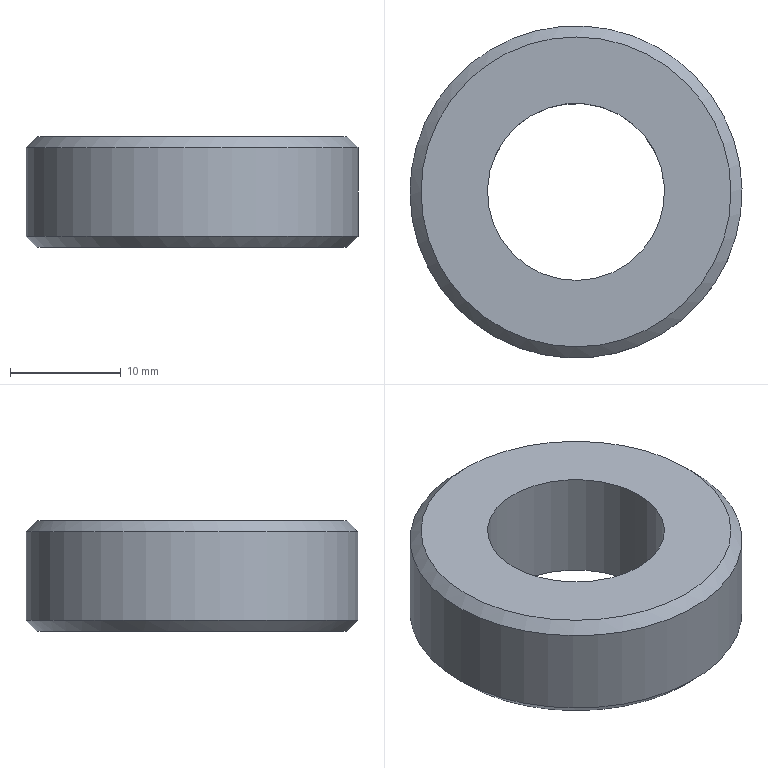Part | STEP file | solid 175 | 1 solid | 6 faces | box 30 x 30 x 10 mm | volume 4966 mm3 | plane 2 | cylinder 2 | cone 2 | commonest cylinder face diameters 16 x1 30 x1